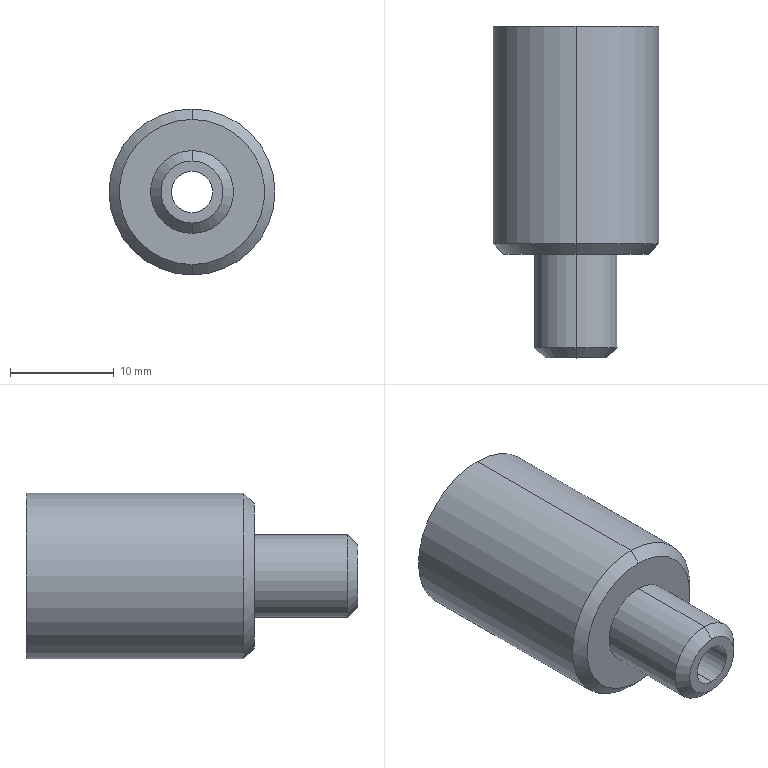Part | SolidWorks | features Chamfer 1, Revolution 1 | 1 solid | 15 faces | box 16 x 32 x 16 mm | volume 3856 mm3 | cylinder 6 | cone 4 | plane 3 | sphere 2 | commonest cylinder face diameters 4 x2 8 x2 16 x2
STEP:
#1=CARTESIAN_POINT('',(0.,10.,-7.));
#2=VERTEX_POINT('',#1);
#3=CARTESIAN_POINT('',(0.,10.,7.));
#4=VERTEX_POINT('',#3);
#5=CARTESIAN_POINT('',(0.,10.,0.));
#6=DIRECTION('',(0.,-1.,0.));
#7=DIRECTION('',(0.,0.,1.));
#8=AXIS2_PLACEMENT_3D('',#5,#6,#7);
#9=CIRCLE('',#8,7.);
#10=EDGE_CURVE('',#2,#4,#9,.T.);
#11=ORIENTED_EDGE('',*,*,#10,.F.);
#12=CARTESIAN_POINT('',(0.,11.,-8.));
#13=VERTEX_POINT('',#12);
#14=CARTESIAN_POINT('',(0.,10.,-7.));
#15=DIRECTION('',(0.,0.7071,-0.7071));
#16=VECTOR('',#15,1000.);
#17=LINE('',#14,#16);
#18=EDGE_CURVE('',#2,#13,#17,.T.);
#19=ORIENTED_EDGE('',*,*,#18,.T.);
#20=CARTESIAN_POINT('',(0.,11.,8.));
#21=VERTEX_POINT('',#20);
#22=CARTESIAN_POINT('',(0.,11.,0.));
#23=DIRECTION('',(0.,1.,0.));
#24=DIRECTION('',(0.,0.,1.));
#25=AXIS2_PLACEMENT_3D('',#22,#23,#24);
#26=CIRCLE('',#25,8.);
#27=EDGE_CURVE('',#21,#13,#26,.T.);
#28=ORIENTED_EDGE('',*,*,#27,.F.);
#29=CARTESIAN_POINT('',(0.,10.,7.));
#30=DIRECTION('',(0.,0.7071,0.7071));
#31=VECTOR('',#30,1000.);
#32=LINE('',#29,#31);
#33=EDGE_CURVE('',#4,#21,#32,.T.);
#34=ORIENTED_EDGE('',*,*,#33,.F.);
#35=EDGE_LOOP('',(#11,#19,#28,#34));
#36=FACE_OUTER_BOUND('',#35,.T.);
#37=CARTESIAN_POINT('',(0.,10.,0.));
#38=DIRECTION('',(0.,1.,0.));
#39=DIRECTION('',(0.,0.,1.));
#40=AXIS2_PLACEMENT_3D('',#37,#38,#39);
#41=CONICAL_SURFACE('',#40,7.,0.7854);
#42=ADVANCED_FACE('',(#36),#41,.T.);
#43=CARTESIAN_POINT('',(0.,0.,-3.));
#44=VERTEX_POINT('',#43);
#45=CARTESIAN_POINT('',(0.,0.,3.));
#46=VERTEX_POINT('',#45);
#47=CARTESIAN_POINT('',(0.,0.,0.));
#48=DIRECTION('',(0.,-1.,0.));
#49=DIRECTION('',(0.,0.,1.));
#50=AXIS2_PLACEMENT_3D('',#47,#48,#49);
#51=CIRCLE('',#50,3.);
#52=EDGE_CURVE('',#44,#46,#51,.T.);
#53=ORIENTED_EDGE('',*,*,#52,.F.);
#54=CARTESIAN_POINT('',(0.,1.,-4.));
#55=VERTEX_POINT('',#54);
#56=CARTESIAN_POINT('',(0.,0.,-3.));
#57=DIRECTION('',(0.,0.7071,-0.7071));
#58=VECTOR('',#57,1000.);
#59=LINE('',#56,#58);
#60=EDGE_CURVE('',#44,#55,#59,.T.);
#61=ORIENTED_EDGE('',*,*,#60,.T.);
#62=CARTESIAN_POINT('',(0.,1.,4.));
#63=VERTEX_POINT('',#62);
#64=CARTESIAN_POINT('',(0.,1.,0.));
#65=DIRECTION('',(0.,1.,0.));
#66=DIRECTION('',(0.,0.,1.));
#67=AXIS2_PLACEMENT_3D('',#64,#65,#66);
#68=CIRCLE('',#67,4.);
#69=EDGE_CURVE('',#63,#55,#68,.T.);
#70=ORIENTED_EDGE('',*,*,#69,.F.);
#71=CARTESIAN_POINT('',(0.,0.,3.));
#72=DIRECTION('',(0.,0.7071,0.7071));
#73=VECTOR('',#72,1000.);
#74=LINE('',#71,#73);
#75=EDGE_CURVE('',#46,#63,#74,.T.);
#76=ORIENTED_EDGE('',*,*,#75,.F.);
#77=EDGE_LOOP('',(#53,#61,#70,#76));
#78=FACE_OUTER_BOUND('',#77,.T.);
#79=CARTESIAN_POINT('',(0.,0.,0.));
#80=DIRECTION('',(0.,1.,0.));
#81=DIRECTION('',(0.,0.,1.));
#82=AXIS2_PLACEMENT_3D('',#79,#80,#81);
#83=CONICAL_SURFACE('',#82,3.,0.7854);
#84=ADVANCED_FACE('',(#78),#83,.T.);
#85=CARTESIAN_POINT('',(0.,32.,-8.));
#86=VERTEX_POINT('',#85);
#87=CARTESIAN_POINT('',(0.,32.,8.));
#88=VERTEX_POINT('',#87);
#89=CARTESIAN_POINT('',(0.,32.,0.));
#90=DIRECTION('',(0.,-1.,0.));
#91=DIRECTION('',(0.,0.,-1.));
#92=AXIS2_PLACEMENT_3D('',#89,#90,#91);
#93=CIRCLE('',#92,8.);
#94=EDGE_CURVE('',#86,#88,#93,.T.);
#95=ORIENTED_EDGE('',*,*,#94,.T.);
#96=CARTESIAN_POINT('',(0.,0.,8.));
#97=DIRECTION('',(0.,-1.,0.));
#98=VECTOR('',#97,1000.);
#99=LINE('',#96,#98);
#100=EDGE_CURVE('',#88,#21,#99,.T.);
#101=ORIENTED_EDGE('',*,*,#100,.T.);
#102=ORIENTED_EDGE('',*,*,#27,.T.);
#103=CARTESIAN_POINT('',(0.,0.,-8.));
#104=DIRECTION('',(0.,-1.,0.));
#105=VECTOR('',#104,1000.);
#106=LINE('',#103,#105);
#107=EDGE_CURVE('',#86,#13,#106,.T.);
#108=ORIENTED_EDGE('',*,*,#107,.F.);
#109=EDGE_LOOP('',(#95,#101,#102,#108));
#110=FACE_OUTER_BOUND('',#109,.T.);
#111=CARTESIAN_POINT('',(0.,0.,0.));
#112=DIRECTION('',(0.,-1.,0.));
#113=DIRECTION('',(0.,0.,-1.));
#114=AXIS2_PLACEMENT_3D('',#111,#112,#113);
#115=CYLINDRICAL_SURFACE('',#114,8.);
#116=ADVANCED_FACE('',(#110),#115,.T.);
#117=CARTESIAN_POINT('',(0.,10.,-4.));
#118=VERTEX_POINT('',#117);
#119=CARTESIAN_POINT('',(0.,10.,4.));
#120=VERTEX_POINT('',#119);
#121=CARTESIAN_POINT('',(0.,10.,0.));
#122=DIRECTION('',(0.,-1.,0.));
#123=DIRECTION('',(0.,0.,-1.));
#124=AXIS2_PLACEMENT_3D('',#121,#122,#123);
#125=CIRCLE('',#124,4.);
#126=EDGE_CURVE('',#118,#120,#125,.T.);
#127=ORIENTED_EDGE('',*,*,#126,.T.);
#128=CARTESIAN_POINT('',(0.,0.,4.));
#129=DIRECTION('',(0.,-1.,0.));
#130=VECTOR('',#129,1000.);
#131=LINE('',#128,#130);
#132=EDGE_CURVE('',#120,#63,#131,.T.);
#133=ORIENTED_EDGE('',*,*,#132,.T.);
#134=ORIENTED_EDGE('',*,*,#69,.T.);
#135=CARTESIAN_POINT('',(0.,0.,-4.));
#136=DIRECTION('',(0.,-1.,0.));
#137=VECTOR('',#136,1000.);
#138=LINE('',#135,#137);
#139=EDGE_CURVE('',#118,#55,#138,.T.);
#140=ORIENTED_EDGE('',*,*,#139,.F.);
#141=EDGE_LOOP('',(#127,#133,#134,#140));
#142=FACE_OUTER_BOUND('',#141,.T.);
#143=CARTESIAN_POINT('',(0.,0.,0.));
#144=DIRECTION('',(0.,-1.,0.));
#145=DIRECTION('',(0.,0.,-1.));
#146=AXIS2_PLACEMENT_3D('',#143,#144,#145);
#147=CYLINDRICAL_SURFACE('',#146,4.);
#148=ADVANCED_FACE('',(#142),#147,.T.);
#149=CARTESIAN_POINT('',(0.,25.292,2.));
#150=VERTEX_POINT('',#149);
#151=CARTESIAN_POINT('',(-2.,25.292,0.));
#152=VERTEX_POINT('',#151);
#153=CARTESIAN_POINT('',(0.,25.292,0.));
#154=DIRECTION('',(0.,-1.,0.));
#155=DIRECTION('',(0.,0.,-1.));
#156=AXIS2_PLACEMENT_3D('',#153,#154,#155);
#157=CIRCLE('',#156,2.);
#158=EDGE_CURVE('',#150,#152,#157,.T.);
#159=ORIENTED_EDGE('',*,*,#158,.F.);
#160=CARTESIAN_POINT('',(0.,0.,2.));
#161=VERTEX_POINT('',#160);
#162=CARTESIAN_POINT('',(0.,0.,2.));
#163=DIRECTION('',(0.,-1.,0.));
#164=VECTOR('',#163,1000.);
#165=LINE('',#162,#164);
#166=EDGE_CURVE('',#150,#161,#165,.T.);
#167=ORIENTED_EDGE('',*,*,#166,.T.);
#168=CARTESIAN_POINT('',(0.,0.,-2.));
#169=VERTEX_POINT('',#168);
#170=CARTESIAN_POINT('',(0.,0.,0.));
#171=DIRECTION('',(0.,-1.,0.));
#172=DIRECTION('',(0.,0.,-1.));
#173=AXIS2_PLACEMENT_3D('',#170,#171,#172);
#174=CIRCLE('',#173,2.);
#175=EDGE_CURVE('',#161,#169,#174,.T.);
#176=ORIENTED_EDGE('',*,*,#175,.T.);
#177=CARTESIAN_POINT('',(0.,25.292,-2.));
#178=VERTEX_POINT('',#177);
#179=CARTESIAN_POINT('',(0.,0.,-2.));
#180=DIRECTION('',(0.,-1.,0.));
#181=VECTOR('',#180,1000.);
#182=LINE('',#179,#181);
#183=EDGE_CURVE('',#178,#169,#182,.T.);
#184=ORIENTED_EDGE('',*,*,#183,.F.);
#185=CARTESIAN_POINT('',(0.,25.292,0.));
#186=DIRECTION('',(0.,-1.,0.));
#187=DIRECTION('',(0.,0.,-1.));
#188=AXIS2_PLACEMENT_3D('',#185,#186,#187);
#189=CIRCLE('',#188,2.);
#190=EDGE_CURVE('',#152,#178,#189,.T.);
#191=ORIENTED_EDGE('',*,*,#190,.F.);
#192=EDGE_LOOP('',(#159,#167,#176,#184,#191));
#193=FACE_OUTER_BOUND('',#192,.T.);
#194=CARTESIAN_POINT('',(0.,0.,0.));
#195=DIRECTION('',(0.,-1.,0.));
#196=DIRECTION('',(0.,0.,-1.));
#197=AXIS2_PLACEMENT_3D('',#194,#195,#196);
#198=CYLINDRICAL_SURFACE('',#197,2.);
#199=ADVANCED_FACE('',(#193),#198,.F.);
#200=CARTESIAN_POINT('',(7.,32.,0.));
#201=VERTEX_POINT('',#200);
#202=CARTESIAN_POINT('',(-7.,32.,0.));
#203=VERTEX_POINT('',#202);
#204=CARTESIAN_POINT('',(0.,32.,0.));
#205=DIRECTION('',(0.,-1.,0.));
#206=DIRECTION('',(0.,0.,-1.));
#207=AXIS2_PLACEMENT_3D('',#204,#205,#206);
#208=CIRCLE('',#207,7.);
#209=EDGE_CURVE('',#201,#203,#208,.T.);
#210=ORIENTED_EDGE('',*,*,#209,.F.);
#211=CARTESIAN_POINT('',(2.,25.292,0.));
#212=VERTEX_POINT('',#211);
#213=CARTESIAN_POINT('',(0.,32.,0.));
#214=DIRECTION('',(0.,0.,-1.));
#215=DIRECTION('',(-1.,0.,0.));
#216=AXIS2_PLACEMENT_3D('',#213,#214,#215);
#217=CIRCLE('',#216,7.);
#218=EDGE_CURVE('',#201,#212,#217,.T.);
#219=ORIENTED_EDGE('',*,*,#218,.T.);
#220=CARTESIAN_POINT('',(0.,25.292,0.));
#221=DIRECTION('',(0.,-1.,0.));
#222=DIRECTION('',(0.,0.,-1.));
#223=AXIS2_PLACEMENT_3D('',#220,#221,#222);
#224=CIRCLE('',#223,2.);
#225=EDGE_CURVE('',#212,#150,#224,.T.);
#226=ORIENTED_EDGE('',*,*,#225,.T.);
#227=ORIENTED_EDGE('',*,*,#158,.T.);
#228=CARTESIAN_POINT('',(0.,32.,0.));
#229=DIRECTION('',(0.,0.,1.));
#230=DIRECTION('',(1.,0.,0.));
#231=AXIS2_PLACEMENT_3D('',#228,#229,#230);
#232=CIRCLE('',#231,7.);
#233=EDGE_CURVE('',#203,#152,#232,.T.);
#234=ORIENTED_EDGE('',*,*,#233,.F.);
#235=EDGE_LOOP('',(#210,#219,#226,#227,#234));
#236=FACE_OUTER_BOUND('',#235,.T.);
#237=CARTESIAN_POINT('',(0.,32.,0.));
#238=DIRECTION('',(0.,0.,-1.));
#239=DIRECTION('',(-1.,0.,0.));
#240=AXIS2_PLACEMENT_3D('',#237,#238,#239);
#241=SPHERICAL_SURFACE('',#240,7.);
#242=ADVANCED_FACE('',(#236),#241,.F.);
#243=ORIENTED_EDGE('',*,*,#218,.F.);
#244=CARTESIAN_POINT('',(0.,32.,0.));
#245=DIRECTION('',(0.,-1.,0.));
#246=DIRECTION('',(0.,0.,-1.));
#247=AXIS2_PLACEMENT_3D('',#244,#245,#246);
#248=CIRCLE('',#247,7.);
#249=EDGE_CURVE('',#203,#201,#248,.T.);
#250=ORIENTED_EDGE('',*,*,#249,.F.);
#251=ORIENTED_EDGE('',*,*,#233,.T.);
#252=ORIENTED_EDGE('',*,*,#190,.T.);
#253=CARTESIAN_POINT('',(0.,25.292,0.));
#254=DIRECTION('',(0.,-1.,0.));
#255=DIRECTION('',(0.,0.,-1.));
#256=AXIS2_PLACEMENT_3D('',#253,#254,#255);
#257=CIRCLE('',#256,2.);
#258=EDGE_CURVE('',#178,#212,#257,.T.);
#259=ORIENTED_EDGE('',*,*,#258,.T.);
#260=EDGE_LOOP('',(#243,#250,#251,#252,#259));
#261=FACE_OUTER_BOUND('',#260,.T.);
#262=CARTESIAN_POINT('',(0.,32.,0.));
#263=DIRECTION('',(0.,0.,-1.));
#264=DIRECTION('',(-1.,0.,0.));
#265=AXIS2_PLACEMENT_3D('',#262,#263,#264);
#266=SPHERICAL_SURFACE('',#265,7.);
#267=ADVANCED_FACE('',(#261),#266,.F.);
#268=ORIENTED_EDGE('',*,*,#166,.F.);
#269=ORIENTED_EDGE('',*,*,#225,.F.);
#270=ORIENTED_EDGE('',*,*,#258,.F.);
#271=ORIENTED_EDGE('',*,*,#183,.T.);
#272=CARTESIAN_POINT('',(0.,0.,0.));
#273=DIRECTION('',(0.,-1.,0.));
#274=DIRECTION('',(0.,0.,-1.));
#275=AXIS2_PLACEMENT_3D('',#272,#273,#274);
#276=CIRCLE('',#275,2.);
#277=EDGE_CURVE('',#169,#161,#276,.T.);
#278=ORIENTED_EDGE('',*,*,#277,.T.);
#279=EDGE_LOOP('',(#268,#269,#270,#271,#278));
#280=FACE_OUTER_BOUND('',#279,.T.);
#281=CARTESIAN_POINT('',(0.,0.,0.));
#282=DIRECTION('',(0.,-1.,0.));
#283=DIRECTION('',(0.,0.,-1.));
#284=AXIS2_PLACEMENT_3D('',#281,#282,#283);
#285=CYLINDRICAL_SURFACE('',#284,2.);
#286=ADVANCED_FACE('',(#280),#285,.F.);
#287=CARTESIAN_POINT('',(0.,0.,0.));
#288=DIRECTION('',(0.,-1.,0.));
#289=DIRECTION('',(0.,0.,1.));
#290=AXIS2_PLACEMENT_3D('',#287,#288,#289);
#291=CIRCLE('',#290,3.);
#292=EDGE_CURVE('',#46,#44,#291,.T.);
#293=ORIENTED_EDGE('',*,*,#292,.T.);
#294=ORIENTED_EDGE('',*,*,#52,.T.);
#295=EDGE_LOOP('',(#293,#294));
#296=FACE_OUTER_BOUND('',#295,.T.);
#297=ORIENTED_EDGE('',*,*,#277,.F.);
#298=ORIENTED_EDGE('',*,*,#175,.F.);
#299=EDGE_LOOP('',(#297,#298));
#300=FACE_BOUND('',#299,.T.);
#301=CARTESIAN_POINT('',(-2.,0.,0.));
#302=DIRECTION('',(0.,1.,0.));
#303=DIRECTION('',(0.,0.,1.));
#304=AXIS2_PLACEMENT_3D('',#301,#302,#303);
#305=PLANE('',#304);
#306=ADVANCED_FACE('',(#296,#300),#305,.F.);
#307=ORIENTED_EDGE('',*,*,#132,.F.);
#308=CARTESIAN_POINT('',(0.,10.,0.));
#309=DIRECTION('',(0.,-1.,0.));
#310=DIRECTION('',(0.,0.,-1.));
#311=AXIS2_PLACEMENT_3D('',#308,#309,#310);
#312=CIRCLE('',#311,4.);
#313=EDGE_CURVE('',#120,#118,#312,.T.);
#314=ORIENTED_EDGE('',*,*,#313,.T.);
#315=ORIENTED_EDGE('',*,*,#139,.T.);
#316=CARTESIAN_POINT('',(0.,1.,0.));
#317=DIRECTION('',(0.,1.,0.));
#318=DIRECTION('',(0.,0.,1.));
#319=AXIS2_PLACEMENT_3D('',#316,#317,#318);
#320=CIRCLE('',#319,4.);
#321=EDGE_CURVE('',#55,#63,#320,.T.);
#322=ORIENTED_EDGE('',*,*,#321,.T.);
#323=EDGE_LOOP('',(#307,#314,#315,#322));
#324=FACE_OUTER_BOUND('',#323,.T.);
#325=CARTESIAN_POINT('',(0.,0.,0.));
#326=DIRECTION('',(0.,-1.,0.));
#327=DIRECTION('',(0.,0.,-1.));
#328=AXIS2_PLACEMENT_3D('',#325,#326,#327);
#329=CYLINDRICAL_SURFACE('',#328,4.);
#330=ADVANCED_FACE('',(#324),#329,.T.);
#331=CARTESIAN_POINT('',(0.,10.,0.));
#332=DIRECTION('',(0.,-1.,0.));
#333=DIRECTION('',(0.,0.,1.));
#334=AXIS2_PLACEMENT_3D('',#331,#332,#333);
#335=CIRCLE('',#334,7.);
#336=EDGE_CURVE('',#4,#2,#335,.T.);
#337=ORIENTED_EDGE('',*,*,#336,.T.);
#338=ORIENTED_EDGE('',*,*,#10,.T.);
#339=EDGE_LOOP('',(#337,#338));
#340=FACE_OUTER_BOUND('',#339,.T.);
#341=ORIENTED_EDGE('',*,*,#126,.F.);
#342=ORIENTED_EDGE('',*,*,#313,.F.);
#343=EDGE_LOOP('',(#341,#342));
#344=FACE_BOUND('',#343,.T.);
#345=CARTESIAN_POINT('',(-8.,10.,0.));
#346=DIRECTION('',(0.,1.,0.));
#347=DIRECTION('',(0.,0.,1.));
#348=AXIS2_PLACEMENT_3D('',#345,#346,#347);
#349=PLANE('',#348);
#350=ADVANCED_FACE('',(#340,#344),#349,.F.);
#351=ORIENTED_EDGE('',*,*,#100,.F.);
#352=CARTESIAN_POINT('',(0.,32.,0.));
#353=DIRECTION('',(0.,-1.,0.));
#354=DIRECTION('',(0.,0.,-1.));
#355=AXIS2_PLACEMENT_3D('',#352,#353,#354);
#356=CIRCLE('',#355,8.);
#357=EDGE_CURVE('',#88,#86,#356,.T.);
#358=ORIENTED_EDGE('',*,*,#357,.T.);
#359=ORIENTED_EDGE('',*,*,#107,.T.);
#360=CARTESIAN_POINT('',(0.,11.,0.));
#361=DIRECTION('',(0.,1.,0.));
#362=DIRECTION('',(0.,0.,1.));
#363=AXIS2_PLACEMENT_3D('',#360,#361,#362);
#364=CIRCLE('',#363,8.);
#365=EDGE_CURVE('',#13,#21,#364,.T.);
#366=ORIENTED_EDGE('',*,*,#365,.T.);
#367=EDGE_LOOP('',(#351,#358,#359,#366));
#368=FACE_OUTER_BOUND('',#367,.T.);
#369=CARTESIAN_POINT('',(0.,0.,0.));
#370=DIRECTION('',(0.,-1.,0.));
#371=DIRECTION('',(0.,0.,-1.));
#372=AXIS2_PLACEMENT_3D('',#369,#370,#371);
#373=CYLINDRICAL_SURFACE('',#372,8.);
#374=ADVANCED_FACE('',(#368),#373,.T.);
#375=ORIENTED_EDGE('',*,*,#94,.F.);
#376=ORIENTED_EDGE('',*,*,#357,.F.);
#377=EDGE_LOOP('',(#375,#376));
#378=FACE_OUTER_BOUND('',#377,.T.);
#379=ORIENTED_EDGE('',*,*,#249,.T.);
#380=ORIENTED_EDGE('',*,*,#209,.T.);
#381=EDGE_LOOP('',(#379,#380));
#382=FACE_BOUND('',#381,.T.);
#383=CARTESIAN_POINT('',(-7.,32.,0.));
#384=DIRECTION('',(0.,-1.,0.));
#385=DIRECTION('',(0.,0.,-1.));
#386=AXIS2_PLACEMENT_3D('',#383,#384,#385);
#387=PLANE('',#386);
#388=ADVANCED_FACE('',(#378,#382),#387,.F.);
#389=ORIENTED_EDGE('',*,*,#60,.F.);
#390=ORIENTED_EDGE('',*,*,#292,.F.);
#391=ORIENTED_EDGE('',*,*,#75,.T.);
#392=ORIENTED_EDGE('',*,*,#321,.F.);
#393=EDGE_LOOP('',(#389,#390,#391,#392));
#394=FACE_OUTER_BOUND('',#393,.T.);
#395=CARTESIAN_POINT('',(0.,0.,0.));
#396=DIRECTION('',(0.,1.,0.));
#397=DIRECTION('',(0.,0.,1.));
#398=AXIS2_PLACEMENT_3D('',#395,#396,#397);
#399=CONICAL_SURFACE('',#398,3.,0.7854);
#400=ADVANCED_FACE('',(#394),#399,.T.);
#401=ORIENTED_EDGE('',*,*,#18,.F.);
#402=ORIENTED_EDGE('',*,*,#336,.F.);
#403=ORIENTED_EDGE('',*,*,#33,.T.);
#404=ORIENTED_EDGE('',*,*,#365,.F.);
#405=EDGE_LOOP('',(#401,#402,#403,#404));
#406=FACE_OUTER_BOUND('',#405,.T.);
#407=CARTESIAN_POINT('',(0.,10.,0.));
#408=DIRECTION('',(0.,1.,0.));
#409=DIRECTION('',(0.,0.,1.));
#410=AXIS2_PLACEMENT_3D('',#407,#408,#409);
#411=CONICAL_SURFACE('',#410,7.,0.7854);
#412=ADVANCED_FACE('',(#406),#411,.T.);
#413=CLOSED_SHELL('',(#42,#84,#116,#148,#199,#242,#267,#286,#306,#330,#350,#374,#388,#400,#412));
#414=MANIFOLD_SOLID_BREP('',#413);
#415=CARTESIAN_POINT('',(0.,0.,0.));
#416=DIRECTION('',(0.,0.,1.));
#417=DIRECTION('',(1.,0.,0.));
#418=AXIS2_PLACEMENT_3D('',#415,#416,#417);
#419=(LENGTH_UNIT()NAMED_UNIT(*)SI_UNIT(.MILLI.,.METRE.));
#420=UNCERTAINTY_MEASURE_WITH_UNIT(LENGTH_MEASURE(0.00001),#419,'','');
#421=(NAMED_UNIT(*)PLANE_ANGLE_UNIT()SI_UNIT($,.RADIAN.));
#422=(NAMED_UNIT(*)SI_UNIT($,.STERADIAN.)SOLID_ANGLE_UNIT());
#423=(GEOMETRIC_REPRESENTATION_CONTEXT(3)GLOBAL_UNCERTAINTY_ASSIGNED_CONTEXT((#420))GLOBAL_UNIT_ASSIGNED_CONTEXT((#419,#421,#422))REPRESENTATION_CONTEXT('',''));
#424=ADVANCED_BREP_SHAPE_REPRESENTATION('',(#414,#418),#423);